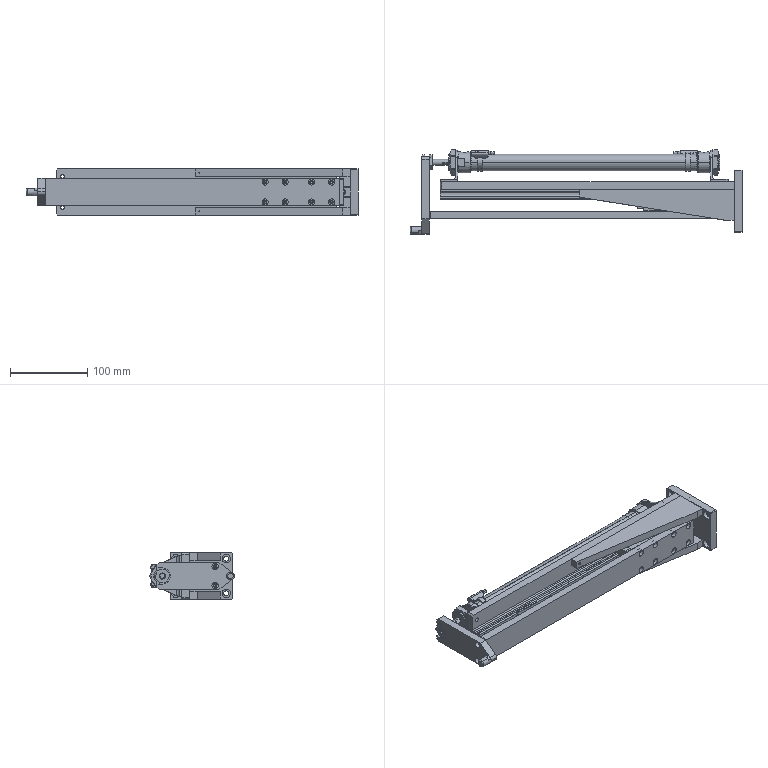Part | SolidWorks | 20 solids | 932 faces | box 429 x 109.5 x 60 mm | volume 759599 mm3 | cylinder 381 | plane 380 | cone 153 | spline 18 | commonest cylinder face diameters 3.3 x62 4.5 x54 8 x44 5.956 x16 7.5 x14 19.6 x14